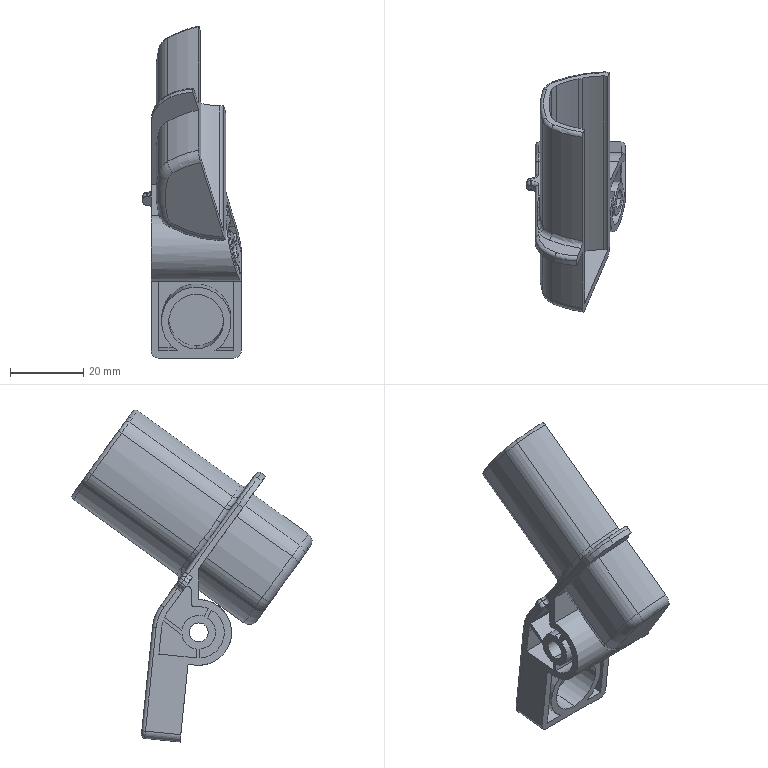Part | SolidWorks | features BaseBody 1 | 1 solid | 160 faces | box 26.902 x 65.621 x 90.738 mm | volume 16180 mm3 | cylinder 71 | plane 55 | torus 25 | spline 7 | sphere 2 | commonest cylinder face diameters 2 x18 9.2 x7 14 x7 20 x5 12 x4 51 x4